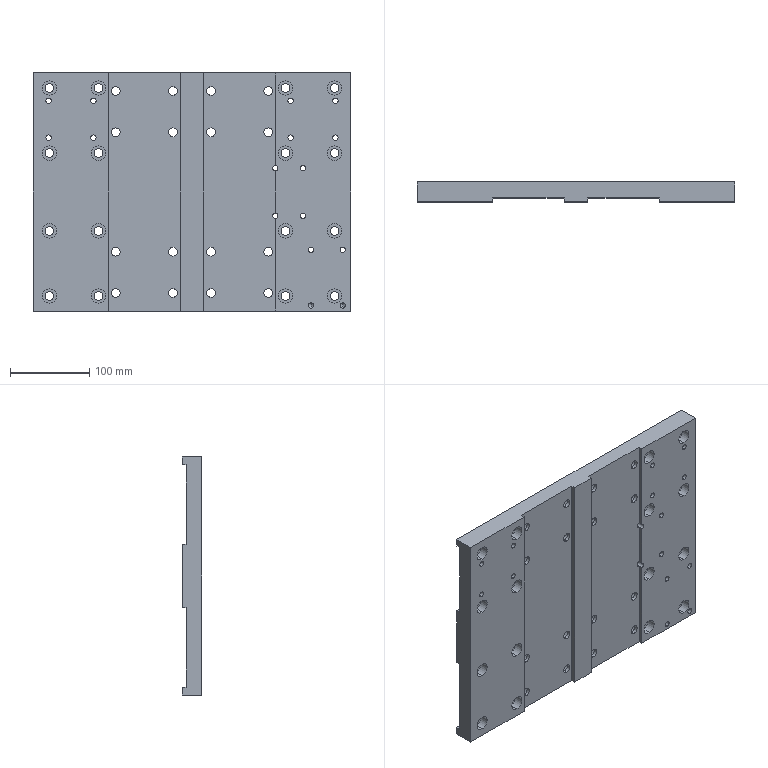Part | STEP file | YCD14007A-08.02.02-Adapter Plate-A3 | 1 solid | 220 faces | box 400 x 25 x 300 mm | volume 2208282 mm3 | cylinder 160 | plane 56 | cone 4 | commonest cylinder face diameters 11 x64 18 x64 6.8 x32